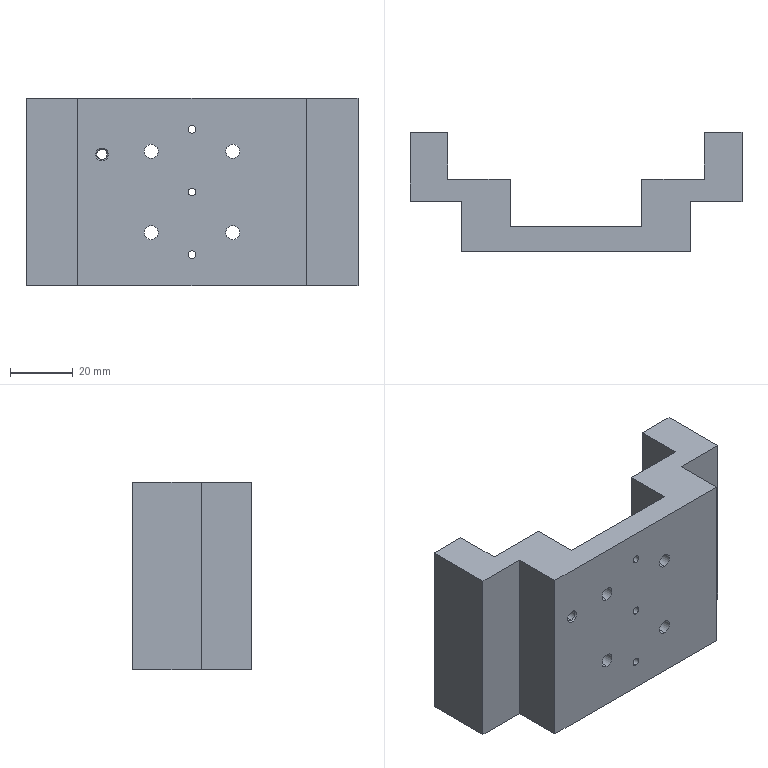Part | SolidWorks | features HoleWzd 7, 3DProfileFeature 4, ICE 4, Chamfer 1, Extrusion 1, LPattern 1, MirrorPattern 1, MoveFace 1 | 1 solid | 97 faces | box 106 x 38 x 60 mm | volume 90816 mm3 | cylinder 48 | cone 26 | plane 23 | commonest cylinder face diameters 2.5 x14 4.2 x12 4.5 x10 8 x8 3.3 x2 11 x2